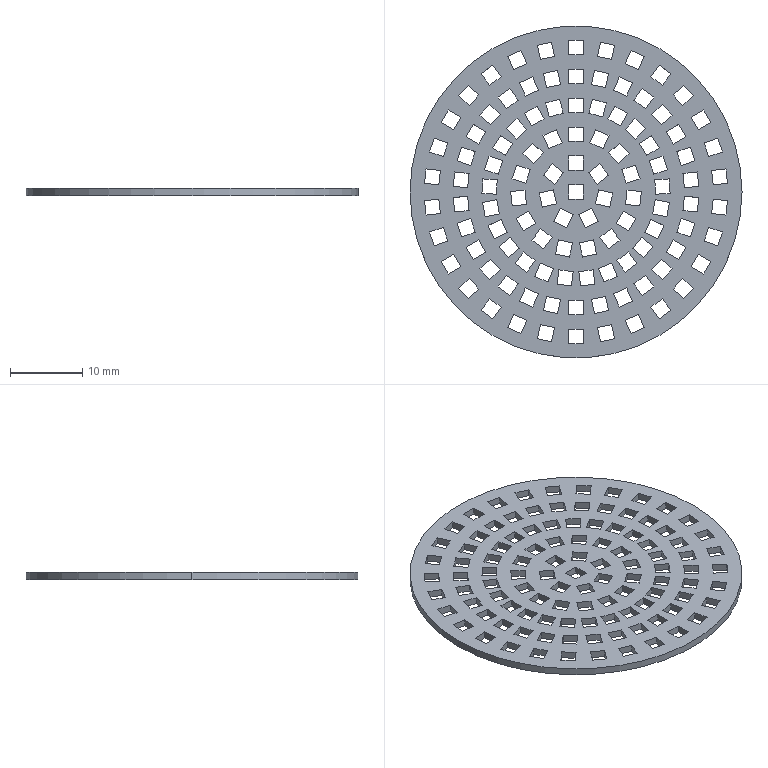Part | SolidWorks | features Extrusion 1 | 1 solid | 436 faces | box 46 x 46 x 1 mm | volume 1230 mm3 | plane 434 | cylinder 2 | commonest cylinder face diameters 46 x2